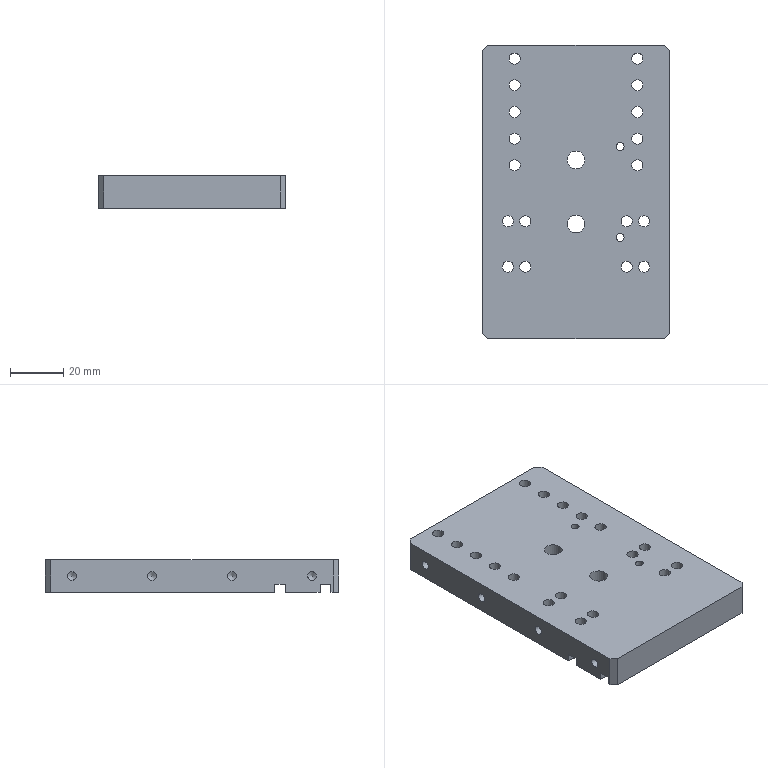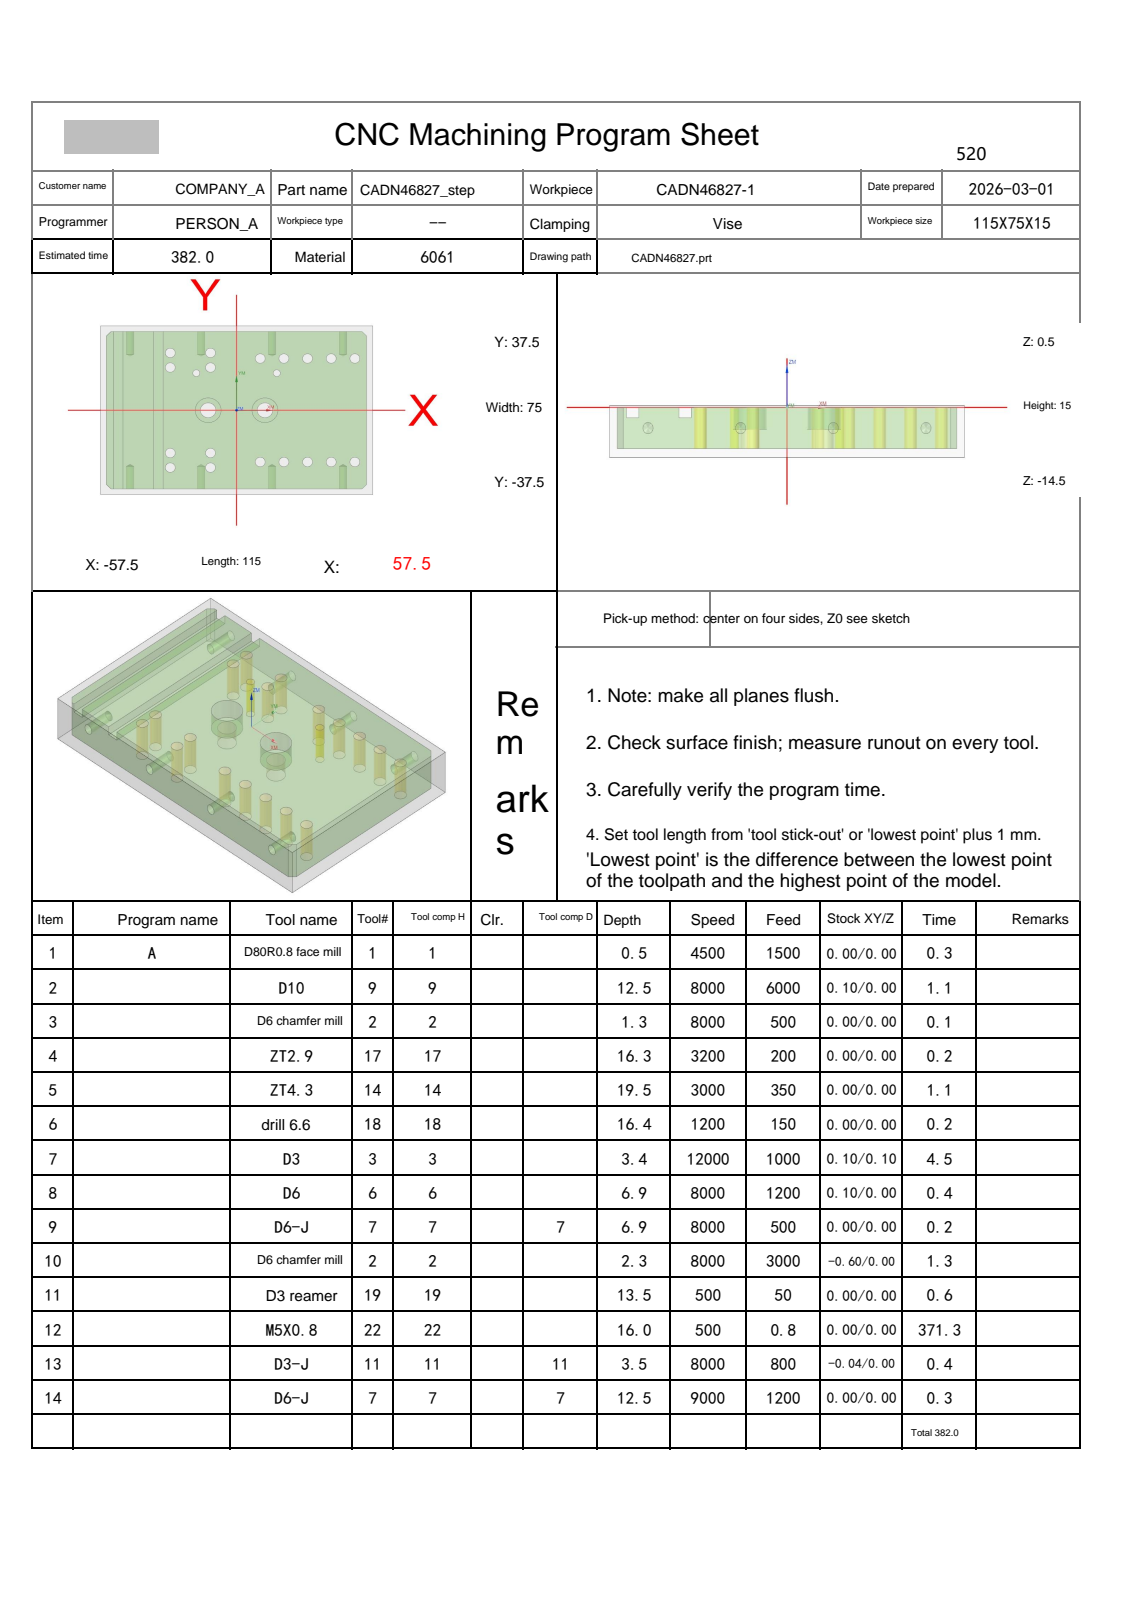NC program | NX | posted by the shop | part box 70 x 110 x 12 mm
Whole program:
%
O0001
(Machine time: 733.44 MIN)
(===Total Tool:12===)
(T1=D80R0.8 face mill D=80. R=0.8 D- H01 Z=0.    )
(T9=D10     D=10.  R=0.   D-  H09 Z=-12.  )
(T2=D6 chamfer mill D=6. R=0. D- H02 Z=-1.8  )
(T17=ZT2.9  D=2.9  DR_a=120 D-  H17 Z=-15.84)
(T14=ZT4.3  D=4.3  DR_a=118 D-  H14 Z=-19.  )
(T18=drill 6.6 D=6.6 DR_a=120 D- H18 Z=-15.91)
(T3=D3      D=3.   R=0.   D-  H03 Z=-2.9  )
(T6=D6      D=6.   R=0.   D-  H06 Z=-6.4  )
(T7=D6-J    D=6.   R=0.   D7  H07 Z=-12.  )
(T19=D3 reamer D=3. DR_a=180 D- H19 Z=-13.  )
(T22=M5X0.8 D=4.2  DR_a=180 D-  H22 Z=-15.5 )
(T11=D3-J   D=3.   R=0.   D11 H11 Z=-3.   )
G80 G90 G17 G49 G40
G91 G28 Z0
M01
N1 T01 M06
(D80R0.8 face mill D=80. R=0.8 H=01 ce=0.00 di=0.00)
G00 G90 G54 X-100. Y25. M03 S4500
G43 H01 Z50.
M08
Z2.
G01 Z0.0 F1500.
X-95.
X95.
Y-25.
X-95.
X-100.
Z2.
G00 Z50.
G91 G28 Z0.0
M05
M09
G91 G28 Z0.0
M01
N2 T09 M06
(D10  D=10. R=0. H=09 ce=0.10 di=0.00)
G00 G90 G54 X0.0 Y-40.1 M03 S8000
G43 H09 Z50.
M08
Z.5
G01 X-53. Z.393 F6000.
G02 X-56.606 Y-38.606 Z.385 I0.0 J5.1
G01 X-58.606 Y-36.606 Z.379
G02 X-60.1 Y-33. Z.371 I3.606 J3.606
G01 Y33. Z.238
G02 X-58.606 Y36.606 Z.23 I5.1 J0.0
G01 X-56.606 Y38.606 Z.224
G02 X-53. Y40.1 Z.216 I3.606 J-3.606
G01 X53. Z.002
G02 X56.606 Y38.606 Z-.006 I0.0 J-5.1
G01 X58.606 Y36.606 Z-.011
G02 X60.1 Y33. Z-.019 I-3.606 J-3.606
G01 Y-33. Z-.152
G02 X58.606 Y-36.606 Z-.161 I-5.1 J0.0
G01 X56.606 Y-38.606 Z-.166
G02 X53. Y-40.1 Z-.174 I-3.606 J3.606
G01 X-53. Z-.388
G02 X-56.606 Y-38.606 Z-.396 I0.0 J5.1
G01 X-58.606 Y-36.606 Z-.402
G02 X-60.1 Y-33. Z-.41 I3.606 J3.606
G01 Y33. Z-.543
G02 X-58.606 Y36.606 Z-.551 I5.1 J0.0
G01 X-56.606 Y38.606 Z-.557
G02 X-53. Y40.1 Z-.565 I3.606 J-3.606
G01 X53. Z-.779
G02 X56.606 Y38.606 Z-.787 I0.0 J-5.1
G01 X58.606 Y36.606 Z-.793
G02 X60.1 Y33. Z-.801 I-3.606 J-3.606
G01 Y-33. Z-.934
G02 X58.606 Y-36.606 Z-.942 I-5.1 J0.0
G01 X56.606 Y-38.606 Z-.948
G02 X53. Y-40.1 Z-.956 I-3.606 J3.606
G01 X-53. Z-1.169
G02 X-56.606 Y-38.606 Z-1.177 I0.0 J5.1
G01 X-58.606 Y-36.606 Z-1.183
G02 X-60.1 Y-33. Z-1.191 I3.606 J3.606
G01 Y33. Z-1.324
G02 X-58.606 Y36.606 Z-1.332 I5.1 J0.0
G01 X-56.606 Y38.606 Z-1.338
G02 X-53. Y40.1 Z-1.346 I3.606 J-3.606
G01 X53. Z-1.56
G02 X56.606 Y38.606 Z-1.568 I0.0 J-5.1
G01 X58.606 Y36.606 Z-1.574
G02 X60.1 Y33. Z-1.582 I-3.606 J-3.606
G01 Y-33. Z-1.715
G02 X58.606 Y-36.606 Z-1.723 I-5.1 J0.0
G01 X56.606 Y-38.606 Z-1.729
G02 X53. Y-40.1 Z-1.737 I-3.606 J3.606
G01 X-53. Z-1.951
G02 X-56.606 Y-38.606 Z-1.959 I0.0 J5.1
G01 X-58.606 Y-36.606 Z-1.964
G02 X-60.1 Y-33. Z-1.973 I3.606 J3.606
G01 Y33. Z-2.106
G02 X-58.606 Y36.606 Z-2.114 I5.1 J0.0
G01 X-56.606 Y38.606 Z-2.119
G02 X-53. Y40.1 Z-2.127 I3.606 J-3.606
G01 X53. Z-2.341
G02 X56.606 Y38.606 Z-2.349 I0.0 J-5.1
G01 X58.606 Y36.606 Z-2.355
G02 X60.1 Y33. Z-2.363 I-3.606 J-3.606
G01 Y-33. Z-2.496
G02 X58.606 Y-36.606 Z-2.504 I-5.1 J0.0
G01 X56.606 Y-38.606 Z-2.51
G02 X53. Y-40.1 Z-2.518 I-3.606 J3.606
G01 X-53. Z-2.732
G02 X-56.606 Y-38.606 Z-2.74 I0.0 J5.1
G01 X-58.606 Y-36.606 Z-2.746
G02 X-60.1 Y-33. Z-2.754 I3.606 J3.606
G01 Y33. Z-2.887
G02 X-58.606 Y36.606 Z-2.895 I5.1 J0.0
G01 X-56.606 Y38.606 Z-2.901
G02 X-53. Y40.1 Z-2.909 I3.606 J-3.606
G01 X53. Z-3.123
G02 X56.606 Y38.606 Z-3.131 I0.0 J-5.1
G01 X58.606 Y36.606 Z-3.136
G02 X60.1 Y33. Z-3.144 I-3.606 J-3.606
G01 Y-33. Z-3.277
G02 X58.606 Y-36.606 Z-3.286 I-5.1 J0.0
G01 X56.606 Y-38.606 Z-3.291
G02 X53. Y-40.1 Z-3.299 I-3.606 J3.606
G01 X-53. Z-3.513
G02 X-56.606 Y-38.606 Z-3.521 I0.0 J5.1
G01 X-58.606 Y-36.606 Z-3.527
G02 X-60.1 Y-33. Z-3.535 I3.606 J3.606
G01 Y33. Z-3.668
G02 X-58.606 Y36.606 Z-3.676 I5.1 J0.0
G01 X-56.606 Y38.606 Z-3.682
G02 X-53. Y40.1 Z-3.69 I3.606 J-3.606
G01 X53. Z-3.904
G02 X56.606 Y38.606 Z-3.912 I0.0 J-5.1
G01 X58.606 Y36.606 Z-3.918
G02 X60.1 Y33. Z-3.926 I-3.606 J-3.606
G01 Y-33. Z-4.059
G02 X58.606 Y-36.606 Z-4.067 I-5.1 J0.0
G01 X56.606 Y-38.606 Z-4.073
G02 X53. Y-40.1 Z-4.081 I-3.606 J3.606
G01 X-53. Z-4.294
G02 X-56.606 Y-38.606 Z-4.302 I0.0 J5.1
G01 X-58.606 Y-36.606 Z-4.308
G02 X-60.1 Y-33. Z-4.316 I3.606 J3.606
G01 Y33. Z-4.449
G02 X-58.606 Y36.606 Z-4.457 I5.1 J0.0
G01 X-56.606 Y38.606 Z-4.463
G02 X-53. Y40.1 Z-4.471 I3.606 J-3.606
G01 X53. Z-4.685
G02 X56.606 Y38.606 Z-4.693 I0.0 J-5.1
G01 X58.606 Y36.606 Z-4.699
G02 X60.1 Y33. Z-4.707 I-3.606 J-3.606
G01 Y-33. Z-4.84
G02 X58.606 Y-36.606 Z-4.848 I-5.1 J0.0
G01 X56.606 Y-38.606 Z-4.854
G02 X53. Y-40.1 Z-4.862 I-3.606 J3.606
G01 X-53. Z-5.076
G02 X-56.606 Y-38.606 Z-5.084 I0.0 J5.1
G01 X-58.606 Y-36.606 Z-5.089
G02 X-60.1 Y-33. Z-5.098 I3.606 J3.606
G01 Y33. Z-5.231
G02 X-58.606 Y36.606 Z-5.239 I5.1 J0.0
G01 X-56.606 Y38.606 Z-5.244
G02 X-53. Y40.1 Z-5.252 I3.606 J-3.606
G01 X53. Z-5.466
G02 X56.606 Y38.606 Z-5.474 I0.0 J-5.1
G01 X58.606 Y36.606 Z-5.48
G02 X60.1 Y33. Z-5.488 I-3.606 J-3.606
G01 Y-33. Z-5.621
G02 X58.606 Y-36.606 Z-5.629 I-5.1 J0.0
G01 X56.606 Y-38.606 Z-5.635
G02 X53. Y-40.1 Z-5.643 I-3.606 J3.606
G01 X-53. Z-5.857
G02 X-56.606 Y-38.606 Z-5.865 I0.0 J5.1
G01 X-58.606 Y-36.606 Z-5.871
G02 X-60.1 Y-33. Z-5.879 I3.606 J3.606
G01 Y33. Z-6.012
G02 X-58.606 Y36.606 Z-6.02 I5.1 J0.0
G01 X-56.606 Y38.606 Z-6.026
G02 X-53. Y40.1 Z-6.034 I3.606 J-3.606
G01 X53. Z-6.248
G02 X56.606 Y38.606 Z-6.256 I0.0 J-5.1
G01 X58.606 Y36.606 Z-6.261
G02 X60.1 Y33. Z-6.269 I-3.606 J-3.606
G01 Y-33. Z-6.402
G02 X58.606 Y-36.606 Z-6.411 I-5.1 J0.0
G01 X56.606 Y-38.606 Z-6.416
G02 X53. Y-40.1 Z-6.424 I-3.606 J3.606
G01 X-53. Z-6.638
G02 X-56.606 Y-38.606 Z-6.646 I0.0 J5.1
G01 X-58.606 Y-36.606 Z-6.652
G02 X-60.1 Y-33. Z-6.66 I3.606 J3.606
G01 Y33. Z-6.793
G02 X-58.606 Y36.606 Z-6.801 I5.1 J0.0
G01 X-56.606 Y38.606 Z-6.807
G02 X-53. Y40.1 Z-6.815 I3.606 J-3.606
G01 X53. Z-7.029
G02 X56.606 Y38.606 Z-7.037 I0.0 J-5.1
G01 X58.606 Y36.606 Z-7.043
G02 X60.1 Y33. Z-7.051 I-3.606 J-3.606
G01 Y-33. Z-7.184
G02 X58.606 Y-36.606 Z-7.192 I-5.1 J0.0
G01 X56.606 Y-38.606 Z-7.198
G02 X53. Y-40.1 Z-7.206 I-3.606 J3.606
G01 X-53. Z-7.419
G02 X-56.606 Y-38.606 Z-7.427 I0.0 J5.1
G01 X-58.606 Y-36.606 Z-7.433
G02 X-60.1 Y-33. Z-7.441 I3.606 J3.606
G01 Y33. Z-7.574
G02 X-58.606 Y36.606 Z-7.582 I5.1 J0.0
G01 X-56.606 Y38.606 Z-7.588
G02 X-53. Y40.1 Z-7.596 I3.606 J-3.606
G01 X53. Z-7.81
G02 X56.606 Y38.606 Z-7.818 I0.0 J-5.1
G01 X58.606 Y36.606 Z-7.824
G02 X60.1 Y33. Z-7.832 I-3.606 J-3.606
G01 Y-33. Z-7.965
G02 X58.606 Y-36.606 Z-7.973 I-5.1 J0.0
G01 X56.606 Y-38.606 Z-7.979
G02 X53. Y-40.1 Z-7.987 I-3.606 J3.606
G01 X-53. Z-8.201
G02 X-56.606 Y-38.606 Z-8.209 I0.0 J5.1
G01 X-58.606 Y-36.606 Z-8.214
G02 X-60.1 Y-33. Z-8.223 I3.606 J3.606
G01 Y33. Z-8.356
G02 X-58.606 Y36.606 Z-8.364 I5.1 J0.0
G01 X-56.606 Y38.606 Z-8.369
G02 X-53. Y40.1 Z-8.377 I3.606 J-3.606
G01 X53. Z-8.591
G02 X56.606 Y38.606 Z-8.599 I0.0 J-5.1
G01 X58.606 Y36.606 Z-8.605
G02 X60.1 Y33. Z-8.613 I-3.606 J-3.606
G01 Y-33. Z-8.746
G02 X58.606 Y-36.606 Z-8.754 I-5.1 J0.0
G01 X56.606 Y-38.606 Z-8.76
G02 X53. Y-40.1 Z-8.768 I-3.606 J3.606
G01 X-53. Z-8.982
G02 X-56.606 Y-38.606 Z-8.99 I0.0 J5.1
G01 X-58.606 Y-36.606 Z-8.996
G02 X-60.1 Y-33. Z-9.004 I3.606 J3.606
G01 Y33. Z-9.137
G02 X-58.606 Y36.606 Z-9.145 I5.1 J0.0
G01 X-56.606 Y38.606 Z-9.151
G02 X-53. Y40.1 Z-9.159 I3.606 J-3.606
G01 X53. Z-9.373
G02 X56.606 Y38.606 Z-9.381 I0.0 J-5.1
G01 X58.606 Y36.606 Z-9.386
G02 X60.1 Y33. Z-9.394 I-3.606 J-3.606
G01 Y-33. Z-9.527
G02 X58.606 Y-36.606 Z-9.536 I-5.1 J0.0
G01 X56.606 Y-38.606 Z-9.541
G02 X53. Y-40.1 Z-9.549 I-3.606 J3.606
G01 X-53. Z-9.763
G02 X-56.606 Y-38.606 Z-9.771 I0.0 J5.1
G01 X-58.606 Y-36.606 Z-9.777
G02 X-60.1 Y-33. Z-9.785 I3.606 J3.606
G01 Y33. Z-9.918
G02 X-58.606 Y36.606 Z-9.926 I5.1 J0.0
G01 X-56.606 Y38.606 Z-9.932
G02 X-53. Y40.1 Z-9.94 I3.606 J-3.606
G01 X53. Z-10.154
G02 X56.606 Y38.606 Z-10.162 I0.0 J-5.1
G01 X58.606 Y36.606 Z-10.168
G02 X60.1 Y33. Z-10.176 I-3.606 J-3.606
G01 Y-33. Z-10.309
G02 X58.606 Y-36.606 Z-10.317 I-5.1 J0.0
G01 X56.606 Y-38.606 Z-10.323
G02 X53. Y-40.1 Z-10.331 I-3.606 J3.606
G01 X-53. Z-10.544
G02 X-56.606 Y-38.606 Z-10.552 I0.0 J5.1
G01 X-58.606 Y-36.606 Z-10.558
G02 X-60.1 Y-33. Z-10.566 I3.606 J3.606
G01 Y33. Z-10.699
G02 X-58.606 Y36.606 Z-10.707 I5.1 J0.0
G01 X-56.606 Y38.606 Z-10.713
G02 X-53. Y40.1 Z-10.721 I3.606 J-3.606
G01 X53. Z-10.935
G02 X56.606 Y38.606 Z-10.943 I0.0 J-5.1
G01 X58.606 Y36.606 Z-10.949
G02 X60.1 Y33. Z-10.957 I-3.606 J-3.606
G01 Y-33. Z-11.09
G02 X58.606 Y-36.606 Z-11.098 I-5.1 J0.0
G01 X56.606 Y-38.606 Z-11.104
G02 X53. Y-40.1 Z-11.112 I-3.606 J3.606
G01 X-53. Z-11.326
G02 X-56.606 Y-38.606 Z-11.334 I0.0 J5.1
G01 X-58.606 Y-36.606 Z-11.339
G02 X-60.1 Y-33. Z-11.348 I3.606 J3.606
G01 Y33. Z-11.481
G02 X-58.606 Y36.606 Z-11.489 I5.1 J0.0
G01 X-56.606 Y38.606 Z-11.494
G02 X-53. Y40.1 Z-11.502 I3.606 J-3.606
G01 X53. Z-11.716
G02 X56.606 Y38.606 Z-11.724 I0.0 J-5.1
G01 X58.606 Y36.606 Z-11.73
G02 X60.1 Y33. Z-11.738 I-3.606 J-3.606
G01 Y-33. Z-11.871
G02 X58.606 Y-36.606 Z-11.879 I-5.1 J0.0
G01 X56.606 Y-38.606 Z-11.885
G02 X53. Y-40.1 Z-11.893 I-3.606 J3.606
G01 X0.0 Z-12.
X-53.
G02 X-56.606 Y-38.606 I0.0 J5.1
G01 X-58.606 Y-36.606
G02 X-60.1 Y-33. I3.606 J3.606
G01 Y33.
G02 X-58.606 Y36.606 I5.1 J0.0
G01 X-56.606 Y38.606
G02 X-53. Y40.1 I3.606 J-3.606
G01 X53.
G02 X56.606 Y38.606 I0.0 J-5.1
G01 X58.606 Y36.606
G02 X60.1 Y33. I-3.606 J-3.606
G01 Y-33.
G02 X58.606 Y-36.606 I-5.1 J0.0
G01 X56.606 Y-38.606
G02 X53. Y-40.1 I-3.606 J3.606
G01 X0.0
X-.5
Z-11.
G00 Z50.
G91 G28 Z0.0
M05
M09
G91 G28 Z0.0
M01
N3 T02 M06
(D6 chamfer mill D=6. R=0. H=02 ce=0.00 di=0.00)
G00 G90 G54 X50. Y23. M03 S8000
G43 H02 Z50.
M08
G98 G81 X50. Y23. Z-.8 R1. F500.
X40.
X30.
X20.
X17. Y16.5
X12. Y0.0
X10. Y23.
X-11. Y25.5
Y19.
X-17. Y16.5
X-28. Y25.5
Y19.
X-12. Y0.0
X-28. Y-19.
Y-25.5
X-11.
Y-19.
X10. Y-23.
X20.
X30.
X40.
X50.
G80
G00 Z50.
G91 G28 Z0.0
M05
M09
G91 G28 Z0.0
M01
N4 T17 M06
(ZT2.9 D=2.9 DR_a=120 H=17)
G00 G90 G54 X17. Y16.5 M03 S3200
G43 H17 Z50.
M08
G98 G83 X17. Y16.5 Z-15.837 R1. F200. Q2.
X-17.
G80
G00 Z50.
G91 G28 Z0.0
M05
M09
G91 G28 Z0.0
M01
N5 T14 M06
(ZT4.3 D=4.3 DR_a=118 H=14)
G00 G90 G54 X50. Y23. M03 S3000
G43 H14 Z50.
M08
G98 G83 X50. Y23. Z-19. R1. F350. Q3.
X40.
X30.
X20.
X10.
X-11. Y19.
Y25.5
X-28.
Y19.
Y-19.
Y-25.5
X-11.
Y-19.
X10. Y-23.
X20.
X30.
X40.
X50.
G80
G00 Z50.
G91 G28 Z0.0
M05
M09
G91 G28 Z0.0
M01
N6 T18 M06
(drill 6.6 D=6.6 DR_a=120 H=18)
G00 G90 G54 X-12. Y0.0 M03 S1200
G43 H18 Z50.
M08
G98 G83 X-12. Y0.0 Z-15.905 R1. F150. Q2.
X12.
G80
G00 Z50.
G91 G28 Z0.0
M05
M09
G91 G28 Z0.0
M01
N7 T03 M06
(D3  D=3. R=0. H=03 ce=0.10 di=0.10)
G00 G90 G54 X-33. Y-39.6 M03 S12000
G43 H03 Z50.
M08
Z.307
G01 Z-.193 F1000.
Y-35.3
X-32.6
Y35.3
X-33.4
Y-35.3
X-33.
X-32.6
Y-35.2
Z.307
G00 Z50.
X-33. Y-39.6
Z.113
G01 Z-.387
Y-35.3
X-32.6
Y35.3
X-33.4
Y-35.3
X-33.
X-32.6
Y-35.2
Z.113
G00 Z.307
X-33. Y-39.6
Z-.08
G01 Z-.58
Y-35.3
X-32.6
Y35.3
X-33.4
Y-35.3
X-33.
X-32.6
Y-35.2
Z-.08
G00 Z.113
X-33. Y-39.6
Z-.273
G01 Z-.773
Y-35.3
X-32.6
Y35.3
X-33.4
Y-35.3
X-33.
X-32.6
Y-35.2
Z-.273
G00 Z-.08
X-33. Y-39.6
Z-.467
G01 Z-.967
Y-35.3
X-32.6
Y35.3
X-33.4
Y-35.3
X-33.
X-32.6
Y-35.2
Z-.467
G00 Z-.273
X-33. Y-39.6
Z-.66
G01 Z-1.16
Y-35.3
X-32.6
Y35.3
X-33.4
Y-35.3
X-33.
X-32.6
Y-35.2
Z-.66
G00 Z-.467
X-33. Y-39.6
Z-.853
G01 Z-1.353
Y-35.3
X-32.6
Y35.3
X-33.4
Y-35.3
X-33.
X-32.6
Y-35.2
Z-.853
G00 Z-.66
X-33. Y-39.6
Z-1.047
G01 Z-1.547
Y-35.3
X-32.6
Y35.3
X-33.4
Y-35.3
X-33.
X-32.6
Y-35.2
Z-1.047
G00 Z-.853
X-33. Y-39.6
Z-1.24
G01 Z-1.74
Y-35.3
X-32.6
Y35.3
X-33.4
Y-35.3
X-33.
X-32.6
Y-35.2
Z-1.24
G00 Z-1.047
X-33. Y-39.6
Z-1.433
G01 Z-1.933
Y-35.3
X-32.6
Y35.3
X-33.4
Y-35.3
X-33.
X-32.6
Y-35.2
Z-1.433
G00 Z-1.24
X-33. Y-39.6
Z-1.627
G01 Z-2.127
Y-35.3
X-32.6
Y35.3
X-33.4
Y-35.3
X-33.
X-32.6
Y-35.2
Z-1.627
G00 Z-1.433
X-33. Y-39.6
Z-1.82
G01 Z-2.32
Y-35.3
X-32.6
Y35.3
X-33.4
Y-35.3
X-33.
X-32.6
Y-35.2
Z-1.82
G00 Z-1.627
X-33. Y-39.6
Z-2.013
G01 Z-2.513
Y-35.3
X-32.6
Y35.3
X-33.4
Y-35.3
X-33.
X-32.6
Y-35.2
Z-2.013
G00 Z-1.82
X-33. Y-39.6
Z-2.207
G01 Z-2.707
Y-35.3
X-32.6
Y35.3
X-33.4
Y-35.3
X-33.
X-32.6
Y-35.2
Z-2.207
G00 Z-2.013
X-33. Y-39.6
Z-2.4
G01 Z-2.9
Y-35.3
X-32.6
Y35.3
X-33.4
Y-35.3
X-33.
X-32.6
Y-35.2
Z-2.4
G00 Z50.
X-50. Y-39.6
Z.307
G01 Z-.193
Y-35.3
X-49.6
Y35.3
X-50.4
Y-35.3
X-50.
X-49.6
Y-35.2
Z.307
G00 Z50.
X-50. Y-39.6
Z.113
G01 Z-.387
Y-35.3
X-49.6
Y35.3
X-50.4
Y-35.3
X-50.
X-49.6
Y-35.2
Z.113
G00 Z.307
X-50. Y-39.6
Z-.08
G01 Z-.58
Y-35.3
X-49.6
Y35.3
X-50.4
Y-35.3
X-50.
X-49.6
Y-35.2
Z-.08
G00 Z.113
X-50. Y-39.6
Z-.273
G01 Z-.773
Y-35.3
X-49.6
Y35.3
X-50.4
Y-35.3
X-50.
X-49.6
Y-35.2
Z-.273
G00 Z-.08
X-50. Y-39.6
Z-.467
G01 Z-.967
Y-35.3
X-49.6
Y35.3
X-50.4
Y-35.3
X-50.
X-49.6
Y-35.2
Z-.467
G00 Z-.273
X-50. Y-39.6
Z-.66
G01 Z-1.16
Y-35.3
X-49.6
Y35.3
X-50.4
Y-35.3
X-50.
X-49.6
Y-35.2
Z-.66
G00 Z-.467
X-50. Y-39.6
Z-.853
G01 Z-1.353
Y-35.3
X-49.6
Y35.3
X-50.4
Y-35.3
X-50.
X-49.6
Y-35.2
Z-.853
G00 Z-.66
X-50. Y-39.6
Z-1.047
G01 Z-1.547
Y-35.3
X-49.6
Y35.3
X-50.4
Y-35.3
X-50.
X-49.6
Y-35.2
Z-1.047
G00 Z-.853
X-50. Y-39.6
Z-1.24
G01 Z-1.74
Y-35.3
X-49.6
Y35.3
X-50.4
Y-35.3
X-50.
X-49.6
Y-35.2
Z-1.24
G00 Z-1.047
X-50. Y-39.6
Z-1.433
G01 Z-1.933
Y-35.3
X-49.6
Y35.3
X-50.4
Y-35.3
X-50.
X-49.6
Y-35.2
Z-1.433
G00 Z-1.24
X-50. Y-39.6
Z-1.627
G01 Z-2.127
Y-35.3
X-49.6
Y35.3
X-50.4
Y-35.3
X-50.
X-49.6
Y-35.2
Z-1.627
G00 Z-1.433
X-50. Y-39.6
Z-1.82
G01 Z-2.32
Y-35.3
X-49.6
Y35.3
X-50.4
Y-35.3
X-50.
X-49.6
Y-35.2
Z-1.82
G00 Z-1.627
X-50. Y-39.6
Z-2.013
G01 Z-2.513
Y-35.3
X-49.6
Y35.3
X-50.4
Y-35.3
X-50.
X-49.6
Y-35.2
Z-2.013
G00 Z-1.82
X-50. Y-39.6
Z-2.207
G01 Z-2.707
Y-35.3
X-49.6
Y35.3
X-50.4
Y-35.3
X-50.
X-49.6
Y-35.2
Z-2.207
G00 Z-2.013
X-50. Y-39.6
Z-2.4
G01 Z-2.9
Y-35.3
X-49.6
Y35.3
X-50.4
Y-35.3
X-50.
X-49.6
Y-35.2
Z-2.4
G00 Z50.
G91 G28 Z0.0
M05
M09
G91 G28 Z0.0
M01
N8 T06 M06
(D6  D=6. R=0. H=06 ce=0.10 di=0.00)
G00 G90 G54 X-12. Y0.0 M03 S8000
G43 H06 Z50.
M08
Z.5
G03 X-10.8 Y1.2 I0.0 J1.2 F1200.
X-12. Y2.4 I-1.2 J0.0
X-12. Y2.4 Z0.0 I0.0 J-2.4
X-12. Y2.4 Z-.5 I0.0 J-2.4
X-12. Y2.4 Z-1. I0.0 J-2.4
X-12. Y2.4 Z-1.5 I0.0 J-2.4
X-12. Y2.4 Z-2. I0.0 J-2.4
X-12. Y2.4 Z-2.5 I0.0 J-2.4
X-12. Y2.4 Z-3. I0.0 J-2.4
X-12. Y2.4 Z-3.5 I0.0 J-2.4
X-12. Y2.4 Z-4. I0.0 J-2.4
X-12. Y2.4 Z-4.5 I0.0 J-2.4
X-12. Y2.4 Z-5. I0.0 J-2.4
X-12. Y2.4 Z-5.5 I0.0 J-2.4
X-12. Y2.4 Z-6. I0.0 J-2.4
X-9.717 Y.742 Z-6.4 I0.0 J-2.4
X-12. Y2.4 I-2.283 J-.742
X-14.4 Y0.0 I0.0 J-2.4
X-12. Y-2.4 I2.4 J0.0
X-9.6 Y0.0 I0.0 J2.4
X-9.717 Y.742 I-2.4 J0.0
X-10.859 Y1.571 I-1.141 J-.371
X-12.059 Y.371 I0.0 J-1.2
X-12. Y0.0 I1.2 J0.0
G00 Z50.
X12.
Z.5
G03 X13.2 Y1.2 I0.0 J1.2
X12. Y2.4 I-1.2 J0.0
X12. Y2.4 Z0.0 I0.0 J-2.4
X12. Y2.4 Z-.5 I0.0 J-2.4
X12. Y2.4 Z-1. I0.0 J-2.4
X12. Y2.4 Z-1.5 I0.0 J-2.4
X12. Y2.4 Z-2. I0.0 J-2.4
X12. Y2.4 Z-2.5 I0.0 J-2.4
X12. Y2.4 Z-3. I0.0 J-2.4
X12. Y2.4 Z-3.5 I0.0 J-2.4
X12. Y2.4 Z-4. I0.0 J-2.4
X12. Y2.4 Z-4.5 I0.0 J-2.4
X12. Y2.4 Z-5. I0.0 J-2.4
X12. Y2.4 Z-5.5 I0.0 J-2.4
X12. Y2.4 Z-6. I0.0 J-2.4
X14.283 Y.742 Z-6.4 I0.0 J-2.4
X12. Y2.4 I-2.283 J-.742
X9.6 Y0.0 I0.0 J-2.4
X12. Y-2.4 I2.4 J0.0
X14.4 Y0.0 I0.0 J2.4
X14.283 Y.742 I-2.4 J0.0
X13.141 Y1.571 I-1.141 J-.371
X11.941 Y.371 I0.0 J-1.2
X12. Y0.0 I1.2 J0.0
G00 Z50.
G91 G28 Z0.0
M05
M09
G91 G28 Z0.0
M01
N9 T07 M06
(D6-J  D=6. R=0. H=07 ce=0.00 di=0.00)
G00 G90 G54 X-12. Y0.0 M03 S8000
G43 H07 Z50.
M08
Z0.0
G41 D07
G01 X-11.803 Y.032 F500.
G03 X-10.758 Y1.258 I-.197 J1.226
X-12. Y2.5 I-1.242 J0.0
X-12. Y2.5 Z-5. I0.0 J-2.5
X-14.456 Y-.468 Z-6.4 I0.0 J-2.5
X-12. Y-2.5 I2.456 J.468
X-9.5 Y0.0 I0.0 J2.5
X-12. Y2.5 I-2.5 J0.0
X-14.5 Y0.0 I0.0 J-2.5
X-14.456 Y-.468 I2.5 J0.0
X-13.236 Y-1.478 I1.22 J.233
X-11.994 Y-.236 I0.0 J1.242
G01 Y-.2
G40 X-12. Y0.0
G00 Z50.
X12.
Z0.0
G41 D07
G01 X12.197 Y.032
G03 X13.242 Y1.258 I-.197 J1.226
X12. Y2.5 I-1.242 J0.0
X12. Y2.5 Z-5. I0.0 J-2.5
X9.544 Y-.468 Z-6.4 I0.0 J-2.5
X12. Y-2.5 I2.456 J.468
X14.5 Y0.0 I0.0 J2.5
X12. Y2.5 I-2.5 J0.0
X9.5 Y0.0 I0.0 J-2.5
X9.544 Y-.468 I2.5 J0.0
X10.764 Y-1.478 I1.22 J.233
X12.006 Y-.236 I0.0 J1.242
G01 Y-.2
G40 X12. Y0.0
G00 Z50.
G91 G28 Z0.0
M05
M09
G91 G28 Z0.0
M01
N10 T02 M06
(D6 chamfer mill D=6. R=0. H=02 ce=0.00 di=0.00)
G00 G90 G54 X11.25 Y-37.128 M03 S8000
G43 H02 Z50.
M08
Z2.099
G01 Z-1.5 F3000.
G03 X11.33 Y-36.828 I-.52 J.3
X11.03 Y-36.308 I-.6 J0.0
G01 X11. Y-36.3
X-31.
G02 X-32.3 Y-35. I0.0 J1.3
G01 Y35.
G02 X-31. Y36.3 I1.3 J0.0
G01 X53.
X53.254 Y36.275
X53.497 Y36.201
X53.722 Y36.081
X53.919 Y35.919
X55.919 Y33.919
X56.081 Y33.722
X56.201 Y33.497
X56.275 Y33.254
X56.3 Y33.
Y-33.
X56.275 Y-33.254
X56.201 Y-33.497
X56.081 Y-33.722
X55.919 Y-33.919
X53.919 Y-35.919
X53.722 Y-36.081
X53.497 Y-36.201
X53.254 Y-36.275
X53. Y-36.3
X11.
X10.97 Y-36.308
G03 X10.67 Y-36.828 I.3 J-.52
X10.75 Y-37.128 I.6 J0.0
G01 Z2.099
G00 Z50.
X-32.872 Y.25
Z2.355
G01 Z-1.5
G03 X-33.172 Y.33 I-.3 J-.52
X-33.692 Y.03 I0.0 J-.6
G01 X-33.7 Y0.0
Y-35.
G02 X-35. Y-36.3 I-1.3 J0.0
G01 X-48.
G02 X-49.3 Y-35. I0.0 J1.3
G01 Y35.
G02 X-48. Y36.3 I1.3 J0.0
G01 X-35.
G02 X-33.7 Y35. I0.0 J-1.3
G01 Y0.0
X-33.692 Y-.03
G03 X-33.172 Y-.33 I.52 J.3
X-32.872 Y-.25 I0.0 J.6
G01 Z2.355
G00 Z50.
X-49.872 Y.25
Z2.355
G01 Z-1.5
G03 X-50.172 Y.33 I-.3 J-.52
X-50.692 Y.03 I0.0 J-.6
G01 X-50.7 Y0.0
Y-35.
G02 X-52. Y-36.3 I-1.3 J0.0
G01 X-53.
X-53.254 Y-36.275
X-53.497 Y-36.201
X-53.722 Y-36.081
X-53.919 Y-35.919
X-55.919 Y-33.919
X-56.081 Y-33.722
X-56.201 Y-33.497
X-56.275 Y-33.254
X-56.3 Y-33.
Y33.
X-56.275 Y33.254
X-56.201 Y33.497
X-56.081 Y33.722
X-55.919 Y33.919
X-53.919 Y35.919
X-53.722 Y36.081
X-53.497 Y36.201
X-53.254 Y36.275
X-53. Y36.3
X-52.
G02 X-50.7 Y35. I0.0 J-1.3
G01 Y0.0
X-50.692 Y-.03
G03 X-50.172 Y-.33 I.52 J.3
X-49.872 Y-.25 I0.0 J.6
G01 Z2.355
G00 Z50.
G00 G90 X17. Y16.5 M03 S8000
Z50.
G98 G81 X17. Y16.5 Z-1.8 R3. F500.
X-17.
G80
G00 Z50.
G00 G90 X50.694 Y23.093 M03 S8000
Z50.
Z-.5
G01 Z-1. F500.
X51.5 Y23.2
G03 X50. Y24.7 I-1.5 J0.0
X48.3 Y23. I0.0 J-1.7
X50. Y21.3 I1.7 J0.0
X51.7 Y23. I0.0 J1.7
X50. Y24.7 I-1.7 J0.0
X48.5 Y23.2 I0.0 J-1.5
G01 X49.306 Y23.093
Z-.5
G00 Z50.
X40.694
Z-.5
G01 Z-1.
X41.5 Y23.2
G03 X40. Y24.7 I-1.5 J0.0
X38.3 Y23. I0.0 J-1.7
X40. Y21.3 I1.7 J0.0
X41.7 Y23. I0.0 J1.7
X40. Y24.7 I-1.7 J0.0
X38.5 Y23.2 I0.0 J-1.5
G01 X39.306 Y23.093
Z-.5
G00 Z50.
X30.694
Z-.5
G01 Z-1.
X31.5 Y23.2
G03 X30. Y24.7 I-1.5 J0.0
X28.3 Y23. I0.0 J-1.7
X30. Y21.3 I1.7 J0.0
X31.7 Y23. I0.0 J1.7
X30. Y24.7 I-1.7 J0.0
X28.5 Y23.2 I0.0 J-1.5
G01 X29.306 Y23.093
Z-.5
G00 Z50.
X20.694
Z-.5
G01 Z-1.
X21.5 Y23.2
G03 X20. Y24.7 I-1.5 J0.0
X18.3 Y23. I0.0 J-1.7
X20. Y21.3 I1.7 J0.0
X21.7 Y23. I0.0 J1.7
X20. Y24.7 I-1.7 J0.0
X18.5 Y23.2 I0.0 J-1.5
G01 X19.306 Y23.093
Z-.5
G00 Z50.
X10.694
Z-.5
G01 Z-1.
X11.5 Y23.2
G03 X10. Y24.7 I-1.5 J0.0
X8.3 Y23. I0.0 J-1.7
X10. Y21.3 I1.7 J0.0
X11.7 Y23. I0.0 J1.7
X10. Y24.7 I-1.7 J0.0
X8.5 Y23.2 I0.0 J-1.5
G01 X9.306 Y23.093
Z-.5
G00 Z50.
X-10.306 Y19.093
Z-.5
G01 Z-1.
X-9.5 Y19.2
G03 X-11. Y20.7 I-1.5 J0.0
X-12.7 Y19. I0.0 J-1.7
X-11. Y17.3 I1.7 J0.0
X-9.3 Y19. I0.0 J1.7
X-11. Y20.7 I-1.7 J0.0
X-12.5 Y19.2 I0.0 J-1.5
G01 X-11.694 Y19.093
Z-.5
G00 Z50.
X-10.306 Y25.593
Z-.5
G01 Z-1.
X-9.5 Y25.7
G03 X-11. Y27.2 I-1.5 J0.0
X-12.7 Y25.5 I0.0 J-1.7
X-11. Y23.8 I1.7 J0.0
X-9.3 Y25.5 I0.0 J1.7
X-11. Y27.2 I-1.7 J0.0
X-12.5 Y25.7 I0.0 J-1.5
G01 X-11.694 Y25.593
Z-.5
G00 Z50.
X-27.306
Z-.5
G01 Z-1.
X-26.5 Y25.7
G03 X-28. Y27.2 I-1.5 J0.0
X-29.7 Y25.5 I0.0 J-1.7
X-28. Y23.8 I1.7 J0.0
X-26.3 Y25.5 I0.0 J1.7
X-28. Y27.2 I-1.7 J0.0
X-29.5 Y25.7 I0.0 J-1.5
G01 X-28.694 Y25.593
Z-.5
G00 Z50.
X-27.306 Y19.093
Z-.5
G01 Z-1.
X-26.5 Y19.2
G03 X-28. Y20.7 I-1.5 J0.0
X-29.7 Y19. I0.0 J-1.7
X-28. Y17.3 I1.7 J0.0
X-26.3 Y19. I0.0 J1.7
X-28. Y20.7 I-1.7 J0.0
X-29.5 Y19.2 I0.0 J-1.5
G01 X-28.694 Y19.093
Z-.5
G00 Z50.
X-27.306 Y-18.907
Z-.5
G01 Z-1.
X-26.5 Y-18.8
G03 X-28. Y-17.3 I-1.5 J0.0
X-29.7 Y-19. I0.0 J-1.7
X-28. Y-20.7 I1.7 J0.0
X-26.3 Y-19. I0.0 J1.7
X-28. Y-17.3 I-1.7 J0.0
X-29.5 Y-18.8 I0.0 J-1.5
G01 X-28.694 Y-18.907
Z-.5
G00 Z50.
X-27.306 Y-25.407
Z-.5
G01 Z-1.
X-26.5 Y-25.3
G03 X-28. Y-23.8 I-1.5 J0.0
X-29.7 Y-25.5 I0.0 J-1.7
X-28. Y-27.2 I1.7 J0.0
X-26.3 Y-25.5 I0.0 J1.7
X-28. Y-23.8 I-1.7 J0.0
X-29.5 Y-25.3 I0.0 J-1.5
G01 X-28.694 Y-25.407
Z-.5
G00 Z50.
X-10.306
Z-.5
G01 Z-1.
X-9.5 Y-25.3
G03 X-11. Y-23.8 I-1.5 J0.0
X-12.7 Y-25.5 I0.0 J-1.7
X-11. Y-27.2 I1.7 J0.0
X-9.3 Y-25.5 I0.0 J1.7
X-11. Y-23.8 I-1.7 J0.0
X-12.5 Y-25.3 I0.0 J-1.5
G01 X-11.694 Y-25.407
Z-.5
G00 Z50.
X-10.306 Y-18.907
Z-.5
G01 Z-1.
X-9.5 Y-18.8
G03 X-11. Y-17.3 I-1.5 J0.0
X-12.7 Y-19. I0.0 J-1.7
X-11. Y-20.7 I1.7 J0.0
X-9.3 Y-19. I0.0 J1.7
X-11. Y-17.3 I-1.7 J0.0
X-12.5 Y-18.8 I0.0 J-1.5
G01 X-11.694 Y-18.907
Z-.5
G00 Z50.
X10.694 Y-22.907
Z-.5
G01 Z-1.
X11.5 Y-22.8
G03 X10. Y-21.3 I-1.5 J0.0
X8.3 Y-23. I0.0 J-1.7
X10. Y-24.7 I1.7 J0.0
X11.7 Y-23. I0.0 J1.7
X10. Y-21.3 I-1.7 J0.0
X8.5 Y-22.8 I0.0 J-1.5
G01 X9.306 Y-22.907
Z-.5
G00 Z50.
X20.694
Z-.5
G01 Z-1.
X21.5 Y-22.8
G03 X20. Y-21.3 I-1.5 J0.0
X18.3 Y-23. I0.0 J-1.7
X20. Y-24.7 I1.7 J0.0
X21.7 Y-23. I0.0 J1.7
X20. Y-21.3 I-1.7 J0.0
X18.5 Y-22.8 I0.0 J-1.5
G01 X19.306 Y-22.907
Z-.5
G00 Z50.
X30.694
Z-.5
G01 Z-1.
X31.5 Y-22.8
G03 X30. Y-21.3 I-1.5 J0.0
X28.3 Y-23. I0.0 J-1.7
X30. Y-24.7 I1.7 J0.0
X31.7 Y-23. I0.0 J1.7
X30. Y-21.3 I-1.7 J0.0
X28.5 Y-22.8 I0.0 J-1.5
G01 X29.306 Y-22.907
Z-.5
G00 Z50.
X40.694
Z-.5
G01 Z-1.
X41.5 Y-22.8
G03 X40. Y-21.3 I-1.5 J0.0
X38.3 Y-23. I0.0 J-1.7
X40. Y-24.7 I1.7 J0.0
X41.7 Y-23. I0.0 J1.7
X40. Y-21.3 I-1.7 J0.0
X38.5 Y-22.8 I0.0 J-1.5
G01 X39.306 Y-22.907
Z-.5
G00 Z50.
X50.694
Z-.5
G01 Z-1.
X51.5 Y-22.8
G03 X50. Y-21.3 I-1.5 J0.0
X48.3 Y-23. I0.0 J-1.7
X50. Y-24.7 I1.7 J0.0
X51.7 Y-23. I0.0 J1.7
X50. Y-21.3 I-1.7 J0.0
X48.5 Y-22.8 I0.0 J-1.5
G01 X49.306 Y-22.907
Z-.5
G00 Z50.
G00 G90 X-16.357 Y2.009 M03 S8000
Z50.
Z2.5
G01 X-16.439 Y1.834 Z2.43 F800.
X-16.595 Y1.399 Z2.261
X-16.708 Y.95 Z2.093
X-16.778 Y.493 Z1.925
X-16.803 Y.031 Z1.756
X-16.784 Y-.431 Z1.588
X-16.72 Y-.89 Z1.419
X-16.612 Y-1.34 Z1.251
X-16.462 Y-1.777 Z1.083
X-16.27 Y-2.198 Z.914
X-16.039 Y-2.599 Z.746
X-15.77 Y-2.976 Z.577
X-15.466 Y-3.325 Z.409
X-15.13 Y-3.643 Z.241
X-14.765 Y-3.927 Z.072
X-14.375 Y-4.175 Z-.096
X-13.962 Y-4.384 Z-.265
X-13.531 Y-4.552 Z-.433
X-13.086 Y-4.679 Z-.601
X-12.631 Y-4.761 Z-.77
X-12.17 Y-4.8 Z-.938
X-12. Z-1.
G03 X-7.2 Y0.0 I0.0 J4.8
X-12. Y4.8 I-4.8 J0.0
X-16.8 Y0.0 I0.0 J-4.8
X-12. Y-4.8 I4.8 J0.0
X-11.501 Y-4.774 I0.0 J4.8
G01 Z1.5
G00 Z50.
X7.643 Y2.009
Z2.5
G01 X7.561 Y1.834 Z2.43
X7.405 Y1.399 Z2.261
X7.292 Y.95 Z2.093
X7.222 Y.493 Z1.925
X7.197 Y.031 Z1.756
X7.216 Y-.431 Z1.588
X7.28 Y-.89 Z1.419
X7.388 Y-1.34 Z1.251
X7.538 Y-1.777 Z1.083
X7.73 Y-2.198 Z.914
X7.961 Y-2.599 Z.746
X8.23 Y-2.976 Z.577
X8.534 Y-3.325 Z.409
X8.87 Y-3.643 Z.241
X9.235 Y-3.927 Z.072
X9.625 Y-4.175 Z-.096
X10.038 Y-4.384 Z-.265
X10.469 Y-4.552 Z-.433
X10.914 Y-4.679 Z-.601
X11.369 Y-4.761 Z-.77
X11.83 Y-4.8 Z-.938
X12. Z-1.
G03 X16.8 Y0.0 I0.0 J4.8
X12. Y4.8 I-4.8 J0.0
X7.2 Y0.0 I0.0 J-4.8
X12. Y-4.8 I4.8 J0.0
X12.499 Y-4.774 I0.0 J4.8
G01 Z1.5
G00 Z50.
G91 G28 Z0.0
M05
M09
G91 G28 Z0.0
M01
N11 T19 M06
(D3 reamer D=3. DR_a=180 H=19)
G00 G90 G54 X17. Y16.5 M03 S500
G43 H19 Z50.
M08
G98 G81 X17. Y16.5 Z-13. R1. F50.
X-17.
G80
G00 Z50.
G91 G28 Z0.0
M05
M09
G91 G28 Z0.0
M01
N12 T22 M06
(M5X0.8 D=4.2 DR_a=180 H=22)
G00 G90 G54 X50. Y23. M03 S500
G43 H22 Z50.
M08
G95
G98 G84 X50. Y23. Z-15.5 R1. F.8 Q3.
X40.
X30.
X20.
X10.
X-11. Y19.
Y25.5
X-28.
Y19.
Y-19.
Y-25.5
X-11.
Y-19.
X10. Y-23.
X20.
X30.
X40.
X50.
G80
G94
G00 Z50.
G91 G28 Z0.0
M05
M09
G91 G28 Z0.0
M01
N13 T11 M06
(D3-J  D=3. R=0. H=11 ce=-0.04 di=0.00)
G00 G90 G54 X-49.54 Y37.56 M03 S8000
G43 H11 Z50.
M08
Z-2.5
G01 Z-3. F800.
G41 D11
Y37.35
G03 X-50.54 Y36.35 I0.0 J-1.
G01 Y-36.35
G03 X-49.54 Y-37.35 I1. J0.0
G01 G40 X-49.44
X-50.56
G41 D11
X-50.46
G03 X-49.46 Y-36.35 I0.0 J1.
G01 Y36.35
G03 X-50.46 Y37.35 I-1. J0.0
G01 Y37.46
G40 Y37.56
Z-2.5
G00 Z50.
X-32.54
Z-2.5
G01 Z-3.
G41 D11
Y37.35
G03 X-33.54 Y36.35 I0.0 J-1.
G01 Y-36.35
G03 X-32.54 Y-37.35 I1. J0.0
G01 G40 X-32.44
X-33.56
G41 D11
X-33.46
G03 X-32.46 Y-36.35 I0.0 J1.
G01 Y36.35
G03 X-33.46 Y37.35 I-1. J0.0
G01 Y37.46
G40 Y37.56
Z-2.5
G00 Z50.
G91 G28 Z0.0
M05
M09
G91 G28 Z0.0
M01
N14 T07 M06
(D6-J  D=6. R=0. H=07 ce=0.00 di=0.00)
G00 G90 G54 X54.017 Y-39.073 M03 S9000
G43 H07 Z50.
M08
Z-11.5
G01 Z-12. F1200.
G41 D07
X53.992 Y-38.875
G03 X53. Y-38. I-.992 J-.125
G01 X-53.
G02 X-55.121 Y-37.121 I0.0 J3.
G01 X-57.121 Y-35.121
G02 X-58. Y-33. I2.121 J2.121
G01 Y33.
G02 X-57.121 Y35.121 I3. J0.0
G01 X-55.121 Y37.121
G02 X-53. Y38. I2.121 J-2.121
G01 X53.
G02 X55.121 Y37.121 I0.0 J-3.
G01 X57.121 Y35.121
G02 X58. Y33. I-2.121 J-2.121
G01 Y-33.
G02 X57.121 Y-35.121 I-3. J0.0
G01 X55.121 Y-37.121
G02 X53. Y-38. I-2.121 J2.121
G01 X52.5
G03 X51.5 Y-39. I0.0 J-1.
G01 G40 Y-39.2
Z-11.5
G00 Z50.
M05
M09
G91 G28 Z0.0
G91 G28 Y0.0
M30
%